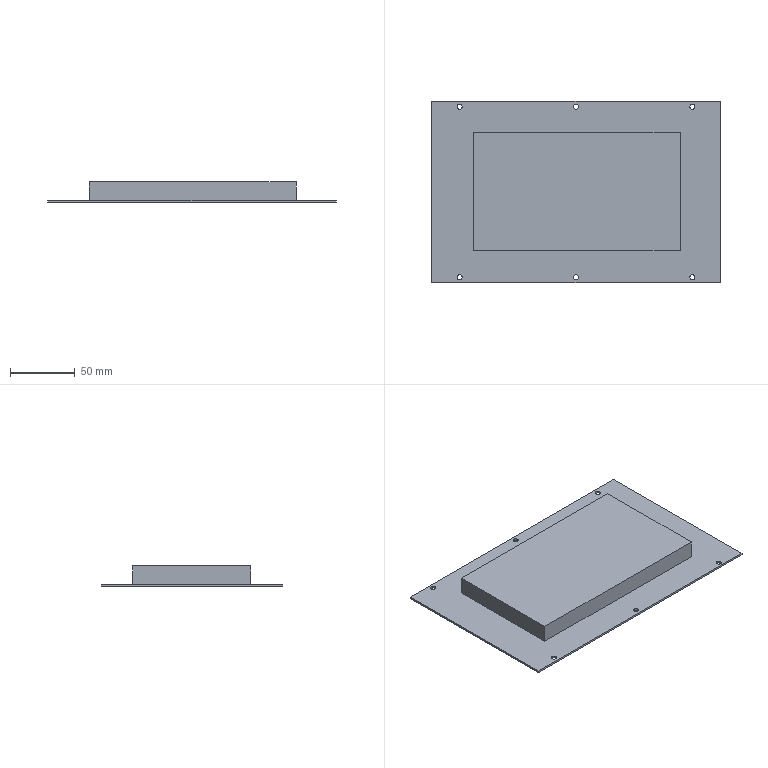Part | STEP file | Q7C1214W | 1 solid | 17 faces | box 223 x 140 x 15.5 mm | volume 251677 mm3 | plane 11 | cylinder 6 | commonest cylinder face diameters 4 x6
STEP:
#1=CARTESIAN_POINT('',(0.,0.,0.));
#2=DIRECTION('',(0.,0.,1.));
#3=DIRECTION('',(1.,0.,0.));
#4=AXIS2_PLACEMENT_3D('',#1,#2,#3);
#5=CARTESIAN_POINT('',(-79.5,46.,1.5));
#6=VERTEX_POINT('',#5);
#7=CARTESIAN_POINT('',(80.5,46.,1.5));
#8=VERTEX_POINT('',#7);
#9=CARTESIAN_POINT('',(-111.5,46.,1.5));
#10=DIRECTION('',(1.,0.,0.));
#11=VECTOR('',#10,1.);
#12=LINE('',#9,#11);
#13=CARTESIAN_POINT('',(-111.5,70.,1.5));
#14=DIRECTION('',(0.,0.,-1.));
#15=DIRECTION('',(-1.,0.,0.));
#16=AXIS2_PLACEMENT_3D('',#13,#14,#15);
#17=PLANE('',#16);
#18=CARTESIAN_POINT('',(0.,-24.));
#19=DIRECTION('',(-1.,0.));
#20=VECTOR('',#19,1.);
#21=LINE('',#18,#20);
#22=(GEOMETRIC_REPRESENTATION_CONTEXT(2)PARAMETRIC_REPRESENTATION_CONTEXT()REPRESENTATION_CONTEXT('',''));
#23=DEFINITIONAL_REPRESENTATION('',(#21),#22);
#24=PCURVE('',#17,#23);
#25=CARTESIAN_POINT('',(80.5,46.,15.5));
#26=DIRECTION('',(0.,1.,0.));
#27=DIRECTION('',(-1.,0.,0.));
#28=AXIS2_PLACEMENT_3D('',#25,#26,#27);
#29=PLANE('',#28);
#30=CARTESIAN_POINT('',(192.,-14.));
#31=DIRECTION('',(-1.,0.));
#32=VECTOR('',#31,1.);
#33=LINE('',#30,#32);
#34=(GEOMETRIC_REPRESENTATION_CONTEXT(2)PARAMETRIC_REPRESENTATION_CONTEXT()REPRESENTATION_CONTEXT('',''));
#35=DEFINITIONAL_REPRESENTATION('',(#33),#34);
#36=PCURVE('',#29,#35);
#37=SURFACE_CURVE('',#12,(#24,#36),.PCURVE_S1.);
#38=EDGE_CURVE('',#6,#8,#37,.T.);
#39=ORIENTED_EDGE('',*,*,#38,.T.);
#40=CARTESIAN_POINT('',(80.5,-45.5,1.5));
#41=VERTEX_POINT('',#40);
#42=CARTESIAN_POINT('',(80.5,70.,1.5));
#43=DIRECTION('',(0.,-1.,0.));
#44=VECTOR('',#43,1.);
#45=LINE('',#42,#44);
#46=CARTESIAN_POINT('',(-192.,0.));
#47=DIRECTION('',(0.,-1.));
#48=VECTOR('',#47,1.);
#49=LINE('',#46,#48);
#50=(GEOMETRIC_REPRESENTATION_CONTEXT(2)PARAMETRIC_REPRESENTATION_CONTEXT()REPRESENTATION_CONTEXT('',''));
#51=DEFINITIONAL_REPRESENTATION('',(#49),#50);
#52=PCURVE('',#17,#51);
#53=CARTESIAN_POINT('',(80.5,46.,15.5));
#54=DIRECTION('',(1.,0.,0.));
#55=DIRECTION('',(0.,1.,0.));
#56=AXIS2_PLACEMENT_3D('',#53,#54,#55);
#57=PLANE('',#56);
#58=CARTESIAN_POINT('',(24.,-14.));
#59=DIRECTION('',(-1.,0.));
#60=VECTOR('',#59,1.);
#61=LINE('',#58,#60);
#62=(GEOMETRIC_REPRESENTATION_CONTEXT(2)PARAMETRIC_REPRESENTATION_CONTEXT()REPRESENTATION_CONTEXT('',''));
#63=DEFINITIONAL_REPRESENTATION('',(#61),#62);
#64=PCURVE('',#57,#63);
#65=SURFACE_CURVE('',#45,(#52,#64),.PCURVE_S1.);
#66=EDGE_CURVE('',#8,#41,#65,.T.);
#67=ORIENTED_EDGE('',*,*,#66,.T.);
#68=CARTESIAN_POINT('',(-79.5,-45.5,1.5));
#69=VERTEX_POINT('',#68);
#70=CARTESIAN_POINT('',(-111.5,-45.5,1.5));
#71=DIRECTION('',(-1.,0.,0.));
#72=VECTOR('',#71,1.);
#73=LINE('',#70,#72);
#74=CARTESIAN_POINT('',(0.,-115.5));
#75=DIRECTION('',(1.,0.));
#76=VECTOR('',#75,1.);
#77=LINE('',#74,#76);
#78=(GEOMETRIC_REPRESENTATION_CONTEXT(2)PARAMETRIC_REPRESENTATION_CONTEXT()REPRESENTATION_CONTEXT('',''));
#79=DEFINITIONAL_REPRESENTATION('',(#77),#78);
#80=PCURVE('',#17,#79);
#81=CARTESIAN_POINT('',(80.5,-45.5,15.5));
#82=DIRECTION('',(0.,-1.,0.));
#83=DIRECTION('',(1.,0.,0.));
#84=AXIS2_PLACEMENT_3D('',#81,#82,#83);
#85=PLANE('',#84);
#86=CARTESIAN_POINT('',(-192.,-14.));
#87=DIRECTION('',(-1.,0.));
#88=VECTOR('',#87,1.);
#89=LINE('',#86,#88);
#90=(GEOMETRIC_REPRESENTATION_CONTEXT(2)PARAMETRIC_REPRESENTATION_CONTEXT()REPRESENTATION_CONTEXT('',''));
#91=DEFINITIONAL_REPRESENTATION('',(#89),#90);
#92=PCURVE('',#85,#91);
#93=SURFACE_CURVE('',#73,(#80,#92),.PCURVE_S1.);
#94=EDGE_CURVE('',#41,#69,#93,.T.);
#95=ORIENTED_EDGE('',*,*,#94,.T.);
#96=CARTESIAN_POINT('',(-79.5,70.,1.5));
#97=DIRECTION('',(0.,1.,0.));
#98=VECTOR('',#97,1.);
#99=LINE('',#96,#98);
#100=CARTESIAN_POINT('',(-32.,0.));
#101=DIRECTION('',(0.,1.));
#102=VECTOR('',#101,1.);
#103=LINE('',#100,#102);
#104=(GEOMETRIC_REPRESENTATION_CONTEXT(2)PARAMETRIC_REPRESENTATION_CONTEXT()REPRESENTATION_CONTEXT('',''));
#105=DEFINITIONAL_REPRESENTATION('',(#103),#104);
#106=PCURVE('',#17,#105);
#107=CARTESIAN_POINT('',(-79.5,46.,15.5));
#108=DIRECTION('',(-1.,0.,0.));
#109=DIRECTION('',(0.,-1.,0.));
#110=AXIS2_PLACEMENT_3D('',#107,#108,#109);
#111=PLANE('',#110);
#112=CARTESIAN_POINT('',(-24.,-14.));
#113=DIRECTION('',(-1.,0.));
#114=VECTOR('',#113,1.);
#115=LINE('',#112,#114);
#116=(GEOMETRIC_REPRESENTATION_CONTEXT(2)PARAMETRIC_REPRESENTATION_CONTEXT()REPRESENTATION_CONTEXT('',''));
#117=DEFINITIONAL_REPRESENTATION('',(#115),#116);
#118=PCURVE('',#111,#117);
#119=SURFACE_CURVE('',#99,(#106,#118),.PCURVE_S1.);
#120=EDGE_CURVE('',#69,#6,#119,.T.);
#121=ORIENTED_EDGE('',*,*,#120,.T.);
#122=EDGE_LOOP('',(#39,#67,#95,#121));
#123=FACE_BOUND('',#122,.T.);
#124=CARTESIAN_POINT('',(2.,-66.,1.5));
#125=VERTEX_POINT('',#124);
#126=CARTESIAN_POINT('',(0.,-66.,1.5));
#127=DIRECTION('',(0.,0.,1.));
#128=DIRECTION('',(1.,0.,0.));
#129=AXIS2_PLACEMENT_3D('',#126,#127,#128);
#130=CIRCLE('',#129,2.);
#131=CARTESIAN_POINT('',(-113.5,-136.));
#132=CARTESIAN_POINT('',(-113.5,-132.536));
#133=CARTESIAN_POINT('',(-110.5,-134.268));
#134=CARTESIAN_POINT('',(-107.5,-136.));
#135=CARTESIAN_POINT('',(-110.5,-137.732));
#136=CARTESIAN_POINT('',(-113.5,-139.464));
#137=CARTESIAN_POINT('',(-113.5,-136.));
#138=(BOUNDED_CURVE()B_SPLINE_CURVE(2,(#131,#132,#133,#134,#135,#136,#137),.UNSPECIFIED.,.T.,.F.)B_SPLINE_CURVE_WITH_KNOTS((1,2,2,2,2,1),(-2.094,0.,2.094,4.189,6.283,8.378),.UNSPECIFIED.)CURVE()GEOMETRIC_REPRESENTATION_ITEM()RATIONAL_B_SPLINE_CURVE((1.,0.5,1.,0.5,1.,0.5,1.))REPRESENTATION_ITEM(''));
#139=(GEOMETRIC_REPRESENTATION_CONTEXT(2)PARAMETRIC_REPRESENTATION_CONTEXT()REPRESENTATION_CONTEXT('',''));
#140=DEFINITIONAL_REPRESENTATION('',(#138),#139);
#141=PCURVE('',#17,#140);
#142=CARTESIAN_POINT('',(0.,-66.,1.5));
#143=DIRECTION('',(0.,0.,-1.));
#144=DIRECTION('',(-1.,0.,0.));
#145=AXIS2_PLACEMENT_3D('',#142,#143,#144);
#146=CYLINDRICAL_SURFACE('',#145,2.);
#147=CARTESIAN_POINT('',(9.425,0.));
#148=DIRECTION('',(-1.,0.));
#149=VECTOR('',#148,1.);
#150=LINE('',#147,#149);
#151=(GEOMETRIC_REPRESENTATION_CONTEXT(2)PARAMETRIC_REPRESENTATION_CONTEXT()REPRESENTATION_CONTEXT('',''));
#152=DEFINITIONAL_REPRESENTATION('',(#150),#151);
#153=PCURVE('',#146,#152);
#154=SURFACE_CURVE('',#130,(#141,#153),.PCURVE_S1.);
#155=EDGE_CURVE('',#125,#125,#154,.T.);
#156=ORIENTED_EDGE('',*,*,#155,.F.);
#157=EDGE_LOOP('',(#156));
#158=FACE_BOUND('',#157,.T.);
#159=CARTESIAN_POINT('',(92.,66.,1.5));
#160=VERTEX_POINT('',#159);
#161=CARTESIAN_POINT('',(90.,66.,1.5));
#162=DIRECTION('',(0.,0.,1.));
#163=DIRECTION('',(1.,0.,0.));
#164=AXIS2_PLACEMENT_3D('',#161,#162,#163);
#165=CIRCLE('',#164,2.);
#166=CARTESIAN_POINT('',(-203.5,-4.));
#167=CARTESIAN_POINT('',(-203.5,-0.5359));
#168=CARTESIAN_POINT('',(-200.5,-2.268));
#169=CARTESIAN_POINT('',(-197.5,-4.));
#170=CARTESIAN_POINT('',(-200.5,-5.732));
#171=CARTESIAN_POINT('',(-203.5,-7.464));
#172=CARTESIAN_POINT('',(-203.5,-4.));
#173=(BOUNDED_CURVE()B_SPLINE_CURVE(2,(#166,#167,#168,#169,#170,#171,#172),.UNSPECIFIED.,.T.,.F.)B_SPLINE_CURVE_WITH_KNOTS((1,2,2,2,2,1),(-2.094,0.,2.094,4.189,6.283,8.378),.UNSPECIFIED.)CURVE()GEOMETRIC_REPRESENTATION_ITEM()RATIONAL_B_SPLINE_CURVE((1.,0.5,1.,0.5,1.,0.5,1.))REPRESENTATION_ITEM(''));
#174=(GEOMETRIC_REPRESENTATION_CONTEXT(2)PARAMETRIC_REPRESENTATION_CONTEXT()REPRESENTATION_CONTEXT('',''));
#175=DEFINITIONAL_REPRESENTATION('',(#173),#174);
#176=PCURVE('',#17,#175);
#177=CARTESIAN_POINT('',(90.,66.,1.5));
#178=DIRECTION('',(0.,0.,-1.));
#179=DIRECTION('',(-1.,0.,0.));
#180=AXIS2_PLACEMENT_3D('',#177,#178,#179);
#181=CYLINDRICAL_SURFACE('',#180,2.);
#182=CARTESIAN_POINT('',(9.425,0.));
#183=DIRECTION('',(-1.,0.));
#184=VECTOR('',#183,1.);
#185=LINE('',#182,#184);
#186=(GEOMETRIC_REPRESENTATION_CONTEXT(2)PARAMETRIC_REPRESENTATION_CONTEXT()REPRESENTATION_CONTEXT('',''));
#187=DEFINITIONAL_REPRESENTATION('',(#185),#186);
#188=PCURVE('',#181,#187);
#189=SURFACE_CURVE('',#165,(#176,#188),.PCURVE_S1.);
#190=EDGE_CURVE('',#160,#160,#189,.T.);
#191=ORIENTED_EDGE('',*,*,#190,.F.);
#192=EDGE_LOOP('',(#191));
#193=FACE_BOUND('',#192,.T.);
#194=CARTESIAN_POINT('',(-88.,66.,1.5));
#195=VERTEX_POINT('',#194);
#196=CARTESIAN_POINT('',(-90.,66.,1.5));
#197=DIRECTION('',(0.,0.,1.));
#198=DIRECTION('',(1.,0.,0.));
#199=AXIS2_PLACEMENT_3D('',#196,#197,#198);
#200=CIRCLE('',#199,2.);
#201=CARTESIAN_POINT('',(-23.5,-4.));
#202=CARTESIAN_POINT('',(-23.5,-0.5359));
#203=CARTESIAN_POINT('',(-20.5,-2.268));
#204=CARTESIAN_POINT('',(-17.5,-4.));
#205=CARTESIAN_POINT('',(-20.5,-5.732));
#206=CARTESIAN_POINT('',(-23.5,-7.464));
#207=CARTESIAN_POINT('',(-23.5,-4.));
#208=(BOUNDED_CURVE()B_SPLINE_CURVE(2,(#201,#202,#203,#204,#205,#206,#207),.UNSPECIFIED.,.T.,.F.)B_SPLINE_CURVE_WITH_KNOTS((1,2,2,2,2,1),(-2.094,0.,2.094,4.189,6.283,8.378),.UNSPECIFIED.)CURVE()GEOMETRIC_REPRESENTATION_ITEM()RATIONAL_B_SPLINE_CURVE((1.,0.5,1.,0.5,1.,0.5,1.))REPRESENTATION_ITEM(''));
#209=(GEOMETRIC_REPRESENTATION_CONTEXT(2)PARAMETRIC_REPRESENTATION_CONTEXT()REPRESENTATION_CONTEXT('',''));
#210=DEFINITIONAL_REPRESENTATION('',(#208),#209);
#211=PCURVE('',#17,#210);
#212=CARTESIAN_POINT('',(-90.,66.,1.5));
#213=DIRECTION('',(0.,0.,-1.));
#214=DIRECTION('',(-1.,0.,0.));
#215=AXIS2_PLACEMENT_3D('',#212,#213,#214);
#216=CYLINDRICAL_SURFACE('',#215,2.);
#217=CARTESIAN_POINT('',(9.425,0.));
#218=DIRECTION('',(-1.,0.));
#219=VECTOR('',#218,1.);
#220=LINE('',#217,#219);
#221=(GEOMETRIC_REPRESENTATION_CONTEXT(2)PARAMETRIC_REPRESENTATION_CONTEXT()REPRESENTATION_CONTEXT('',''));
#222=DEFINITIONAL_REPRESENTATION('',(#220),#221);
#223=PCURVE('',#216,#222);
#224=SURFACE_CURVE('',#200,(#211,#223),.PCURVE_S1.);
#225=EDGE_CURVE('',#195,#195,#224,.T.);
#226=ORIENTED_EDGE('',*,*,#225,.F.);
#227=EDGE_LOOP('',(#226));
#228=FACE_BOUND('',#227,.T.);
#229=CARTESIAN_POINT('',(-111.5,70.,1.5));
#230=VERTEX_POINT('',#229);
#231=CARTESIAN_POINT('',(-111.5,-70.,1.5));
#232=VERTEX_POINT('',#231);
#233=CARTESIAN_POINT('',(-111.5,-70.,1.5));
#234=DIRECTION('',(0.,-1.,0.));
#235=VECTOR('',#234,1.);
#236=LINE('',#233,#235);
#237=CARTESIAN_POINT('',(0.,-140.));
#238=DIRECTION('',(0.,-1.));
#239=VECTOR('',#238,1.);
#240=LINE('',#237,#239);
#241=(GEOMETRIC_REPRESENTATION_CONTEXT(2)PARAMETRIC_REPRESENTATION_CONTEXT()REPRESENTATION_CONTEXT('',''));
#242=DEFINITIONAL_REPRESENTATION('',(#240),#241);
#243=PCURVE('',#17,#242);
#244=CARTESIAN_POINT('',(-111.5,-70.,1.5));
#245=DIRECTION('',(1.,0.,0.));
#246=DIRECTION('',(0.,0.,-1.));
#247=AXIS2_PLACEMENT_3D('',#244,#245,#246);
#248=PLANE('',#247);
#249=CARTESIAN_POINT('',(0.,0.));
#250=DIRECTION('',(0.,-1.));
#251=VECTOR('',#250,1.);
#252=LINE('',#249,#251);
#253=(GEOMETRIC_REPRESENTATION_CONTEXT(2)PARAMETRIC_REPRESENTATION_CONTEXT()REPRESENTATION_CONTEXT('',''));
#254=DEFINITIONAL_REPRESENTATION('',(#252),#253);
#255=PCURVE('',#248,#254);
#256=SURFACE_CURVE('',#236,(#243,#255),.PCURVE_S1.);
#257=EDGE_CURVE('',#230,#232,#256,.T.);
#258=ORIENTED_EDGE('',*,*,#257,.T.);
#259=CARTESIAN_POINT('',(111.5,-70.,1.5));
#260=VERTEX_POINT('',#259);
#261=CARTESIAN_POINT('',(-111.5,-70.,1.5));
#262=DIRECTION('',(1.,0.,0.));
#263=VECTOR('',#262,1.);
#264=LINE('',#261,#263);
#265=CARTESIAN_POINT('',(0.,-140.));
#266=DIRECTION('',(-1.,0.));
#267=VECTOR('',#266,1.);
#268=LINE('',#265,#267);
#269=(GEOMETRIC_REPRESENTATION_CONTEXT(2)PARAMETRIC_REPRESENTATION_CONTEXT()REPRESENTATION_CONTEXT('',''));
#270=DEFINITIONAL_REPRESENTATION('',(#268),#269);
#271=PCURVE('',#17,#270);
#272=CARTESIAN_POINT('',(-111.5,-70.,1.5));
#273=DIRECTION('',(0.,1.,0.));
#274=DIRECTION('',(0.,0.,1.));
#275=AXIS2_PLACEMENT_3D('',#272,#273,#274);
#276=PLANE('',#275);
#277=CARTESIAN_POINT('',(0.,0.));
#278=DIRECTION('',(0.,1.));
#279=VECTOR('',#278,1.);
#280=LINE('',#277,#279);
#281=(GEOMETRIC_REPRESENTATION_CONTEXT(2)PARAMETRIC_REPRESENTATION_CONTEXT()REPRESENTATION_CONTEXT('',''));
#282=DEFINITIONAL_REPRESENTATION('',(#280),#281);
#283=PCURVE('',#276,#282);
#284=SURFACE_CURVE('',#264,(#271,#283),.PCURVE_S1.);
#285=EDGE_CURVE('',#232,#260,#284,.T.);
#286=ORIENTED_EDGE('',*,*,#285,.T.);
#287=CARTESIAN_POINT('',(111.5,70.,1.5));
#288=VERTEX_POINT('',#287);
#289=CARTESIAN_POINT('',(111.5,-70.,1.5));
#290=DIRECTION('',(0.,1.,0.));
#291=VECTOR('',#290,1.);
#292=LINE('',#289,#291);
#293=CARTESIAN_POINT('',(-223.,-140.));
#294=DIRECTION('',(0.,1.));
#295=VECTOR('',#294,1.);
#296=LINE('',#293,#295);
#297=(GEOMETRIC_REPRESENTATION_CONTEXT(2)PARAMETRIC_REPRESENTATION_CONTEXT()REPRESENTATION_CONTEXT('',''));
#298=DEFINITIONAL_REPRESENTATION('',(#296),#297);
#299=PCURVE('',#17,#298);
#300=CARTESIAN_POINT('',(111.5,-70.,1.5));
#301=DIRECTION('',(-1.,0.,0.));
#302=DIRECTION('',(0.,0.,1.));
#303=AXIS2_PLACEMENT_3D('',#300,#301,#302);
#304=PLANE('',#303);
#305=CARTESIAN_POINT('',(0.,0.));
#306=DIRECTION('',(0.,1.));
#307=VECTOR('',#306,1.);
#308=LINE('',#305,#307);
#309=(GEOMETRIC_REPRESENTATION_CONTEXT(2)PARAMETRIC_REPRESENTATION_CONTEXT()REPRESENTATION_CONTEXT('',''));
#310=DEFINITIONAL_REPRESENTATION('',(#308),#309);
#311=PCURVE('',#304,#310);
#312=SURFACE_CURVE('',#292,(#299,#311),.PCURVE_S1.);
#313=EDGE_CURVE('',#260,#288,#312,.T.);
#314=ORIENTED_EDGE('',*,*,#313,.T.);
#315=CARTESIAN_POINT('',(-111.5,70.,1.5));
#316=DIRECTION('',(-1.,0.,0.));
#317=VECTOR('',#316,1.);
#318=LINE('',#315,#317);
#319=CARTESIAN_POINT('',(0.,0.));
#320=DIRECTION('',(1.,0.));
#321=VECTOR('',#320,1.);
#322=LINE('',#319,#321);
#323=(GEOMETRIC_REPRESENTATION_CONTEXT(2)PARAMETRIC_REPRESENTATION_CONTEXT()REPRESENTATION_CONTEXT('',''));
#324=DEFINITIONAL_REPRESENTATION('',(#322),#323);
#325=PCURVE('',#17,#324);
#326=CARTESIAN_POINT('',(-111.5,70.,1.5));
#327=DIRECTION('',(0.,-1.,0.));
#328=DIRECTION('',(0.,0.,-1.));
#329=AXIS2_PLACEMENT_3D('',#326,#327,#328);
#330=PLANE('',#329);
#331=CARTESIAN_POINT('',(0.,0.));
#332=DIRECTION('',(0.,-1.));
#333=VECTOR('',#332,1.);
#334=LINE('',#331,#333);
#335=(GEOMETRIC_REPRESENTATION_CONTEXT(2)PARAMETRIC_REPRESENTATION_CONTEXT()REPRESENTATION_CONTEXT('',''));
#336=DEFINITIONAL_REPRESENTATION('',(#334),#335);
#337=PCURVE('',#330,#336);
#338=SURFACE_CURVE('',#318,(#325,#337),.PCURVE_S1.);
#339=EDGE_CURVE('',#288,#230,#338,.T.);
#340=ORIENTED_EDGE('',*,*,#339,.T.);
#341=EDGE_LOOP('',(#258,#286,#314,#340));
#342=FACE_BOUND('',#341,.T.);
#343=CARTESIAN_POINT('',(2.,66.,1.5));
#344=VERTEX_POINT('',#343);
#345=CARTESIAN_POINT('',(0.,66.,1.5));
#346=DIRECTION('',(0.,0.,1.));
#347=DIRECTION('',(1.,0.,0.));
#348=AXIS2_PLACEMENT_3D('',#345,#346,#347);
#349=CIRCLE('',#348,2.);
#350=CARTESIAN_POINT('',(-113.5,-4.));
#351=CARTESIAN_POINT('',(-113.5,-0.5359));
#352=CARTESIAN_POINT('',(-110.5,-2.268));
#353=CARTESIAN_POINT('',(-107.5,-4.));
#354=CARTESIAN_POINT('',(-110.5,-5.732));
#355=CARTESIAN_POINT('',(-113.5,-7.464));
#356=CARTESIAN_POINT('',(-113.5,-4.));
#357=(BOUNDED_CURVE()B_SPLINE_CURVE(2,(#350,#351,#352,#353,#354,#355,#356),.UNSPECIFIED.,.T.,.F.)B_SPLINE_CURVE_WITH_KNOTS((1,2,2,2,2,1),(-2.094,0.,2.094,4.189,6.283,8.378),.UNSPECIFIED.)CURVE()GEOMETRIC_REPRESENTATION_ITEM()RATIONAL_B_SPLINE_CURVE((1.,0.5,1.,0.5,1.,0.5,1.))REPRESENTATION_ITEM(''));
#358=(GEOMETRIC_REPRESENTATION_CONTEXT(2)PARAMETRIC_REPRESENTATION_CONTEXT()REPRESENTATION_CONTEXT('',''));
#359=DEFINITIONAL_REPRESENTATION('',(#357),#358);
#360=PCURVE('',#17,#359);
#361=CARTESIAN_POINT('',(0.,66.,1.5));
#362=DIRECTION('',(0.,0.,-1.));
#363=DIRECTION('',(-1.,0.,0.));
#364=AXIS2_PLACEMENT_3D('',#361,#362,#363);
#365=CYLINDRICAL_SURFACE('',#364,2.);
#366=CARTESIAN_POINT('',(9.425,0.));
#367=DIRECTION('',(-1.,0.));
#368=VECTOR('',#367,1.);
#369=LINE('',#366,#368);
#370=(GEOMETRIC_REPRESENTATION_CONTEXT(2)PARAMETRIC_REPRESENTATION_CONTEXT()REPRESENTATION_CONTEXT('',''));
#371=DEFINITIONAL_REPRESENTATION('',(#369),#370);
#372=PCURVE('',#365,#371);
#373=SURFACE_CURVE('',#349,(#360,#372),.PCURVE_S1.);
#374=EDGE_CURVE('',#344,#344,#373,.T.);
#375=ORIENTED_EDGE('',*,*,#374,.F.);
#376=EDGE_LOOP('',(#375));
#377=FACE_BOUND('',#376,.T.);
#378=CARTESIAN_POINT('',(-88.,-66.,1.5));
#379=VERTEX_POINT('',#378);
#380=CARTESIAN_POINT('',(-90.,-66.,1.5));
#381=DIRECTION('',(0.,0.,1.));
#382=DIRECTION('',(1.,0.,0.));
#383=AXIS2_PLACEMENT_3D('',#380,#381,#382);
#384=CIRCLE('',#383,2.);
#385=CARTESIAN_POINT('',(-23.5,-136.));
#386=CARTESIAN_POINT('',(-23.5,-132.536));
#387=CARTESIAN_POINT('',(-20.5,-134.268));
#388=CARTESIAN_POINT('',(-17.5,-136.));
#389=CARTESIAN_POINT('',(-20.5,-137.732));
#390=CARTESIAN_POINT('',(-23.5,-139.464));
#391=CARTESIAN_POINT('',(-23.5,-136.));
#392=(BOUNDED_CURVE()B_SPLINE_CURVE(2,(#385,#386,#387,#388,#389,#390,#391),.UNSPECIFIED.,.T.,.F.)B_SPLINE_CURVE_WITH_KNOTS((1,2,2,2,2,1),(-2.094,0.,2.094,4.189,6.283,8.378),.UNSPECIFIED.)CURVE()GEOMETRIC_REPRESENTATION_ITEM()RATIONAL_B_SPLINE_CURVE((1.,0.5,1.,0.5,1.,0.5,1.))REPRESENTATION_ITEM(''));
#393=(GEOMETRIC_REPRESENTATION_CONTEXT(2)PARAMETRIC_REPRESENTATION_CONTEXT()REPRESENTATION_CONTEXT('',''));
#394=DEFINITIONAL_REPRESENTATION('',(#392),#393);
#395=PCURVE('',#17,#394);
#396=CARTESIAN_POINT('',(-90.,-66.,1.5));
#397=DIRECTION('',(0.,0.,-1.));
#398=DIRECTION('',(-1.,0.,0.));
#399=AXIS2_PLACEMENT_3D('',#396,#397,#398);
#400=CYLINDRICAL_SURFACE('',#399,2.);
#401=CARTESIAN_POINT('',(9.425,0.));
#402=DIRECTION('',(-1.,0.));
#403=VECTOR('',#402,1.);
#404=LINE('',#401,#403);
#405=(GEOMETRIC_REPRESENTATION_CONTEXT(2)PARAMETRIC_REPRESENTATION_CONTEXT()REPRESENTATION_CONTEXT('',''));
#406=DEFINITIONAL_REPRESENTATION('',(#404),#405);
#407=PCURVE('',#400,#406);
#408=SURFACE_CURVE('',#384,(#395,#407),.PCURVE_S1.);
#409=EDGE_CURVE('',#379,#379,#408,.T.);
#410=ORIENTED_EDGE('',*,*,#409,.F.);
#411=EDGE_LOOP('',(#410));
#412=FACE_BOUND('',#411,.T.);
#413=CARTESIAN_POINT('',(92.,-66.,1.5));
#414=VERTEX_POINT('',#413);
#415=CARTESIAN_POINT('',(90.,-66.,1.5));
#416=DIRECTION('',(0.,0.,1.));
#417=DIRECTION('',(1.,0.,0.));
#418=AXIS2_PLACEMENT_3D('',#415,#416,#417);
#419=CIRCLE('',#418,2.);
#420=CARTESIAN_POINT('',(-203.5,-136.));
#421=CARTESIAN_POINT('',(-203.5,-132.536));
#422=CARTESIAN_POINT('',(-200.5,-134.268));
#423=CARTESIAN_POINT('',(-197.5,-136.));
#424=CARTESIAN_POINT('',(-200.5,-137.732));
#425=CARTESIAN_POINT('',(-203.5,-139.464));
#426=CARTESIAN_POINT('',(-203.5,-136.));
#427=(BOUNDED_CURVE()B_SPLINE_CURVE(2,(#420,#421,#422,#423,#424,#425,#426),.UNSPECIFIED.,.T.,.F.)B_SPLINE_CURVE_WITH_KNOTS((1,2,2,2,2,1),(-2.094,0.,2.094,4.189,6.283,8.378),.UNSPECIFIED.)CURVE()GEOMETRIC_REPRESENTATION_ITEM()RATIONAL_B_SPLINE_CURVE((1.,0.5,1.,0.5,1.,0.5,1.))REPRESENTATION_ITEM(''));
#428=(GEOMETRIC_REPRESENTATION_CONTEXT(2)PARAMETRIC_REPRESENTATION_CONTEXT()REPRESENTATION_CONTEXT('',''));
#429=DEFINITIONAL_REPRESENTATION('',(#427),#428);
#430=PCURVE('',#17,#429);
#431=CARTESIAN_POINT('',(90.,-66.,1.5));
#432=DIRECTION('',(0.,0.,-1.));
#433=DIRECTION('',(-1.,0.,0.));
#434=AXIS2_PLACEMENT_3D('',#431,#432,#433);
#435=CYLINDRICAL_SURFACE('',#434,2.);
#436=CARTESIAN_POINT('',(9.425,0.));
#437=DIRECTION('',(-1.,0.));
#438=VECTOR('',#437,1.);
#439=LINE('',#436,#438);
#440=(GEOMETRIC_REPRESENTATION_CONTEXT(2)PARAMETRIC_REPRESENTATION_CONTEXT()REPRESENTATION_CONTEXT('',''));
#441=DEFINITIONAL_REPRESENTATION('',(#439),#440);
#442=PCURVE('',#435,#441);
#443=SURFACE_CURVE('',#419,(#430,#442),.PCURVE_S1.);
#444=EDGE_CURVE('',#414,#414,#443,.T.);
#445=ORIENTED_EDGE('',*,*,#444,.F.);
#446=EDGE_LOOP('',(#445));
#447=FACE_BOUND('',#446,.T.);
#448=ADVANCED_FACE('',(#123,#158,#193,#228,#342,#377,#412,#447),#17,.F.);
#449=CARTESIAN_POINT('',(2.,-66.,0.));
#450=VERTEX_POINT('',#449);
#451=CARTESIAN_POINT('',(0.,-66.,0.));
#452=DIRECTION('',(0.,0.,1.));
#453=DIRECTION('',(1.,0.,0.));
#454=AXIS2_PLACEMENT_3D('',#451,#452,#453);
#455=CIRCLE('',#454,2.);
#456=CARTESIAN_POINT('',(-111.5,70.,0.));
#457=DIRECTION('',(0.,0.,-1.));
#458=DIRECTION('',(-1.,0.,0.));
#459=AXIS2_PLACEMENT_3D('',#456,#457,#458);
#460=PLANE('',#459);
#461=CARTESIAN_POINT('',(-113.5,-136.));
#462=CARTESIAN_POINT('',(-113.5,-132.536));
#463=CARTESIAN_POINT('',(-110.5,-134.268));
#464=CARTESIAN_POINT('',(-107.5,-136.));
#465=CARTESIAN_POINT('',(-110.5,-137.732));
#466=CARTESIAN_POINT('',(-113.5,-139.464));
#467=CARTESIAN_POINT('',(-113.5,-136.));
#468=(BOUNDED_CURVE()B_SPLINE_CURVE(2,(#461,#462,#463,#464,#465,#466,#467),.UNSPECIFIED.,.T.,.F.)B_SPLINE_CURVE_WITH_KNOTS((1,2,2,2,2,1),(-2.094,0.,2.094,4.189,6.283,8.378),.UNSPECIFIED.)CURVE()GEOMETRIC_REPRESENTATION_ITEM()RATIONAL_B_SPLINE_CURVE((1.,0.5,1.,0.5,1.,0.5,1.))REPRESENTATION_ITEM(''));
#469=(GEOMETRIC_REPRESENTATION_CONTEXT(2)PARAMETRIC_REPRESENTATION_CONTEXT()REPRESENTATION_CONTEXT('',''));
#470=DEFINITIONAL_REPRESENTATION('',(#468),#469);
#471=PCURVE('',#460,#470);
#472=CARTESIAN_POINT('',(9.425,1.5));
#473=DIRECTION('',(-1.,0.));
#474=VECTOR('',#473,1.);
#475=LINE('',#472,#474);
#476=(GEOMETRIC_REPRESENTATION_CONTEXT(2)PARAMETRIC_REPRESENTATION_CONTEXT()REPRESENTATION_CONTEXT('',''));
#477=DEFINITIONAL_REPRESENTATION('',(#475),#476);
#478=PCURVE('',#146,#477);
#479=SURFACE_CURVE('',#455,(#471,#478),.PCURVE_S1.);
#480=EDGE_CURVE('',#450,#450,#479,.T.);
#481=ORIENTED_EDGE('',*,*,#480,.T.);
#482=EDGE_LOOP('',(#481));
#483=FACE_BOUND('',#482,.T.);
#484=CARTESIAN_POINT('',(92.,66.,0.));
#485=VERTEX_POINT('',#484);
#486=CARTESIAN_POINT('',(90.,66.,0.));
#487=DIRECTION('',(0.,0.,1.));
#488=DIRECTION('',(1.,0.,0.));
#489=AXIS2_PLACEMENT_3D('',#486,#487,#488);
#490=CIRCLE('',#489,2.);
#491=CARTESIAN_POINT('',(-203.5,-4.));
#492=CARTESIAN_POINT('',(-203.5,-0.5359));
#493=CARTESIAN_POINT('',(-200.5,-2.268));
#494=CARTESIAN_POINT('',(-197.5,-4.));
#495=CARTESIAN_POINT('',(-200.5,-5.732));
#496=CARTESIAN_POINT('',(-203.5,-7.464));
#497=CARTESIAN_POINT('',(-203.5,-4.));
#498=(BOUNDED_CURVE()B_SPLINE_CURVE(2,(#491,#492,#493,#494,#495,#496,#497),.UNSPECIFIED.,.T.,.F.)B_SPLINE_CURVE_WITH_KNOTS((1,2,2,2,2,1),(-2.094,0.,2.094,4.189,6.283,8.378),.UNSPECIFIED.)CURVE()GEOMETRIC_REPRESENTATION_ITEM()RATIONAL_B_SPLINE_CURVE((1.,0.5,1.,0.5,1.,0.5,1.))REPRESENTATION_ITEM(''));
#499=(GEOMETRIC_REPRESENTATION_CONTEXT(2)PARAMETRIC_REPRESENTATION_CONTEXT()REPRESENTATION_CONTEXT('',''));
#500=DEFINITIONAL_REPRESENTATION('',(#498),#499);
#501=PCURVE('',#460,#500);
#502=CARTESIAN_POINT('',(9.425,1.5));
#503=DIRECTION('',(-1.,0.));
#504=VECTOR('',#503,1.);
#505=LINE('',#502,#504);
#506=(GEOMETRIC_REPRESENTATION_CONTEXT(2)PARAMETRIC_REPRESENTATION_CONTEXT()REPRESENTATION_CONTEXT('',''));
#507=DEFINITIONAL_REPRESENTATION('',(#505),#506);
#508=PCURVE('',#181,#507);
#509=SURFACE_CURVE('',#490,(#501,#508),.PCURVE_S1.);
#510=EDGE_CURVE('',#485,#485,#509,.T.);
#511=ORIENTED_EDGE('',*,*,#510,.T.);
#512=EDGE_LOOP('',(#511));
#513=FACE_BOUND('',#512,.T.);
#514=CARTESIAN_POINT('',(-88.,66.,0.));
#515=VERTEX_POINT('',#514);
#516=CARTESIAN_POINT('',(-90.,66.,0.));
#517=DIRECTION('',(0.,0.,1.));
#518=DIRECTION('',(1.,0.,0.));
#519=AXIS2_PLACEMENT_3D('',#516,#517,#518);
#520=CIRCLE('',#519,2.);
#521=CARTESIAN_POINT('',(-23.5,-4.));
#522=CARTESIAN_POINT('',(-23.5,-0.5359));
#523=CARTESIAN_POINT('',(-20.5,-2.268));
#524=CARTESIAN_POINT('',(-17.5,-4.));
#525=CARTESIAN_POINT('',(-20.5,-5.732));
#526=CARTESIAN_POINT('',(-23.5,-7.464));
#527=CARTESIAN_POINT('',(-23.5,-4.));
#528=(BOUNDED_CURVE()B_SPLINE_CURVE(2,(#521,#522,#523,#524,#525,#526,#527),.UNSPECIFIED.,.T.,.F.)B_SPLINE_CURVE_WITH_KNOTS((1,2,2,2,2,1),(-2.094,0.,2.094,4.189,6.283,8.378),.UNSPECIFIED.)CURVE()GEOMETRIC_REPRESENTATION_ITEM()RATIONAL_B_SPLINE_CURVE((1.,0.5,1.,0.5,1.,0.5,1.))REPRESENTATION_ITEM(''));
#529=(GEOMETRIC_REPRESENTATION_CONTEXT(2)PARAMETRIC_REPRESENTATION_CONTEXT()REPRESENTATION_CONTEXT('',''));
#530=DEFINITIONAL_REPRESENTATION('',(#528),#529);
#531=PCURVE('',#460,#530);
#532=CARTESIAN_POINT('',(9.425,1.5));
#533=DIRECTION('',(-1.,0.));
#534=VECTOR('',#533,1.);
#535=LINE('',#532,#534);
#536=(GEOMETRIC_REPRESENTATION_CONTEXT(2)PARAMETRIC_REPRESENTATION_CONTEXT()REPRESENTATION_CONTEXT('',''));
#537=DEFINITIONAL_REPRESENTATION('',(#535),#536);
#538=PCURVE('',#216,#537);
#539=SURFACE_CURVE('',#520,(#531,#538),.PCURVE_S1.);
#540=EDGE_CURVE('',#515,#515,#539,.T.);
#541=ORIENTED_EDGE('',*,*,#540,.T.);
#542=EDGE_LOOP('',(#541));
#543=FACE_BOUND('',#542,.T.);
#544=CARTESIAN_POINT('',(-111.5,70.,0.));
#545=VERTEX_POINT('',#544);
#546=CARTESIAN_POINT('',(-111.5,-70.,0.));
#547=VERTEX_POINT('',#546);
#548=CARTESIAN_POINT('',(-111.5,-70.,0.));
#549=DIRECTION('',(0.,-1.,0.));
#550=VECTOR('',#549,1.);
#551=LINE('',#548,#550);
#552=CARTESIAN_POINT('',(0.,-140.));
#553=DIRECTION('',(0.,-1.));
#554=VECTOR('',#553,1.);
#555=LINE('',#552,#554);
#556=(GEOMETRIC_REPRESENTATION_CONTEXT(2)PARAMETRIC_REPRESENTATION_CONTEXT()REPRESENTATION_CONTEXT('',''));
#557=DEFINITIONAL_REPRESENTATION('',(#555),#556);
#558=PCURVE('',#460,#557);
#559=CARTESIAN_POINT('',(1.5,0.));
#560=DIRECTION('',(0.,-1.));
#561=VECTOR('',#560,1.);
#562=LINE('',#559,#561);
#563=(GEOMETRIC_REPRESENTATION_CONTEXT(2)PARAMETRIC_REPRESENTATION_CONTEXT()REPRESENTATION_CONTEXT('',''));
#564=DEFINITIONAL_REPRESENTATION('',(#562),#563);
#565=PCURVE('',#248,#564);
#566=SURFACE_CURVE('',#551,(#558,#565),.PCURVE_S1.);
#567=EDGE_CURVE('',#545,#547,#566,.T.);
#568=ORIENTED_EDGE('',*,*,#567,.F.);
#569=CARTESIAN_POINT('',(111.5,70.,0.));
#570=VERTEX_POINT('',#569);
#571=CARTESIAN_POINT('',(-111.5,70.,0.));
#572=DIRECTION('',(-1.,0.,0.));
#573=VECTOR('',#572,1.);
#574=LINE('',#571,#573);
#575=CARTESIAN_POINT('',(0.,0.));
#576=DIRECTION('',(1.,0.));
#577=VECTOR('',#576,1.);
#578=LINE('',#575,#577);
#579=(GEOMETRIC_REPRESENTATION_CONTEXT(2)PARAMETRIC_REPRESENTATION_CONTEXT()REPRESENTATION_CONTEXT('',''));
#580=DEFINITIONAL_REPRESENTATION('',(#578),#579);
#581=PCURVE('',#460,#580);
#582=CARTESIAN_POINT('',(1.5,0.));
#583=DIRECTION('',(0.,-1.));
#584=VECTOR('',#583,1.);
#585=LINE('',#582,#584);
#586=(GEOMETRIC_REPRESENTATION_CONTEXT(2)PARAMETRIC_REPRESENTATION_CONTEXT()REPRESENTATION_CONTEXT('',''));
#587=DEFINITIONAL_REPRESENTATION('',(#585),#586);
#588=PCURVE('',#330,#587);
#589=SURFACE_CURVE('',#574,(#581,#588),.PCURVE_S1.);
#590=EDGE_CURVE('',#570,#545,#589,.T.);
#591=ORIENTED_EDGE('',*,*,#590,.F.);
#592=CARTESIAN_POINT('',(111.5,-70.,0.));
#593=VERTEX_POINT('',#592);
#594=CARTESIAN_POINT('',(111.5,-70.,0.));
#595=DIRECTION('',(0.,1.,0.));
#596=VECTOR('',#595,1.);
#597=LINE('',#594,#596);
#598=CARTESIAN_POINT('',(-223.,-140.));
#599=DIRECTION('',(0.,1.));
#600=VECTOR('',#599,1.);
#601=LINE('',#598,#600);
#602=(GEOMETRIC_REPRESENTATION_CONTEXT(2)PARAMETRIC_REPRESENTATION_CONTEXT()REPRESENTATION_CONTEXT('',''));
#603=DEFINITIONAL_REPRESENTATION('',(#601),#602);
#604=PCURVE('',#460,#603);
#605=CARTESIAN_POINT('',(-1.5,0.));
#606=DIRECTION('',(0.,1.));
#607=VECTOR('',#606,1.);
#608=LINE('',#605,#607);
#609=(GEOMETRIC_REPRESENTATION_CONTEXT(2)PARAMETRIC_REPRESENTATION_CONTEXT()REPRESENTATION_CONTEXT('',''));
#610=DEFINITIONAL_REPRESENTATION('',(#608),#609);
#611=PCURVE('',#304,#610);
#612=SURFACE_CURVE('',#597,(#604,#611),.PCURVE_S1.);
#613=EDGE_CURVE('',#593,#570,#612,.T.);
#614=ORIENTED_EDGE('',*,*,#613,.F.);
#615=CARTESIAN_POINT('',(-111.5,-70.,0.));
#616=DIRECTION('',(1.,0.,0.));
#617=VECTOR('',#616,1.);
#618=LINE('',#615,#617);
#619=CARTESIAN_POINT('',(0.,-140.));
#620=DIRECTION('',(-1.,0.));
#621=VECTOR('',#620,1.);
#622=LINE('',#619,#621);
#623=(GEOMETRIC_REPRESENTATION_CONTEXT(2)PARAMETRIC_REPRESENTATION_CONTEXT()REPRESENTATION_CONTEXT('',''));
#624=DEFINITIONAL_REPRESENTATION('',(#622),#623);
#625=PCURVE('',#460,#624);
#626=CARTESIAN_POINT('',(-1.5,0.));
#627=DIRECTION('',(0.,1.));
#628=VECTOR('',#627,1.);
#629=LINE('',#626,#628);
#630=(GEOMETRIC_REPRESENTATION_CONTEXT(2)PARAMETRIC_REPRESENTATION_CONTEXT()REPRESENTATION_CONTEXT('',''));
#631=DEFINITIONAL_REPRESENTATION('',(#629),#630);
#632=PCURVE('',#276,#631);
#633=SURFACE_CURVE('',#618,(#625,#632),.PCURVE_S1.);
#634=EDGE_CURVE('',#547,#593,#633,.T.);
#635=ORIENTED_EDGE('',*,*,#634,.F.);
#636=EDGE_LOOP('',(#568,#591,#614,#635));
#637=FACE_BOUND('',#636,.T.);
#638=CARTESIAN_POINT('',(2.,66.,0.));
#639=VERTEX_POINT('',#638);
#640=CARTESIAN_POINT('',(0.,66.,0.));
#641=DIRECTION('',(0.,0.,1.));
#642=DIRECTION('',(1.,0.,0.));
#643=AXIS2_PLACEMENT_3D('',#640,#641,#642);
#644=CIRCLE('',#643,2.);
#645=CARTESIAN_POINT('',(-113.5,-4.));
#646=CARTESIAN_POINT('',(-113.5,-0.5359));
#647=CARTESIAN_POINT('',(-110.5,-2.268));
#648=CARTESIAN_POINT('',(-107.5,-4.));
#649=CARTESIAN_POINT('',(-110.5,-5.732));
#650=CARTESIAN_POINT('',(-113.5,-7.464));
#651=CARTESIAN_POINT('',(-113.5,-4.));
#652=(BOUNDED_CURVE()B_SPLINE_CURVE(2,(#645,#646,#647,#648,#649,#650,#651),.UNSPECIFIED.,.T.,.F.)B_SPLINE_CURVE_WITH_KNOTS((1,2,2,2,2,1),(-2.094,0.,2.094,4.189,6.283,8.378),.UNSPECIFIED.)CURVE()GEOMETRIC_REPRESENTATION_ITEM()RATIONAL_B_SPLINE_CURVE((1.,0.5,1.,0.5,1.,0.5,1.))REPRESENTATION_ITEM(''));
#653=(GEOMETRIC_REPRESENTATION_CONTEXT(2)PARAMETRIC_REPRESENTATION_CONTEXT()REPRESENTATION_CONTEXT('',''));
#654=DEFINITIONAL_REPRESENTATION('',(#652),#653);
#655=PCURVE('',#460,#654);
#656=CARTESIAN_POINT('',(9.425,1.5));
#657=DIRECTION('',(-1.,0.));
#658=VECTOR('',#657,1.);
#659=LINE('',#656,#658);
#660=(GEOMETRIC_REPRESENTATION_CONTEXT(2)PARAMETRIC_REPRESENTATION_CONTEXT()REPRESENTATION_CONTEXT('',''));
#661=DEFINITIONAL_REPRESENTATION('',(#659),#660);
#662=PCURVE('',#365,#661);
#663=SURFACE_CURVE('',#644,(#655,#662),.PCURVE_S1.);
#664=EDGE_CURVE('',#639,#639,#663,.T.);
#665=ORIENTED_EDGE('',*,*,#664,.T.);
#666=EDGE_LOOP('',(#665));
#667=FACE_BOUND('',#666,.T.);
#668=CARTESIAN_POINT('',(-88.,-66.,0.));
#669=VERTEX_POINT('',#668);
#670=CARTESIAN_POINT('',(-90.,-66.,0.));
#671=DIRECTION('',(0.,0.,1.));
#672=DIRECTION('',(1.,0.,0.));
#673=AXIS2_PLACEMENT_3D('',#670,#671,#672);
#674=CIRCLE('',#673,2.);
#675=CARTESIAN_POINT('',(-23.5,-136.));
#676=CARTESIAN_POINT('',(-23.5,-132.536));
#677=CARTESIAN_POINT('',(-20.5,-134.268));
#678=CARTESIAN_POINT('',(-17.5,-136.));
#679=CARTESIAN_POINT('',(-20.5,-137.732));
#680=CARTESIAN_POINT('',(-23.5,-139.464));
#681=CARTESIAN_POINT('',(-23.5,-136.));
#682=(BOUNDED_CURVE()B_SPLINE_CURVE(2,(#675,#676,#677,#678,#679,#680,#681),.UNSPECIFIED.,.T.,.F.)B_SPLINE_CURVE_WITH_KNOTS((1,2,2,2,2,1),(-2.094,0.,2.094,4.189,6.283,8.378),.UNSPECIFIED.)CURVE()GEOMETRIC_REPRESENTATION_ITEM()RATIONAL_B_SPLINE_CURVE((1.,0.5,1.,0.5,1.,0.5,1.))REPRESENTATION_ITEM(''));
#683=(GEOMETRIC_REPRESENTATION_CONTEXT(2)PARAMETRIC_REPRESENTATION_CONTEXT()REPRESENTATION_CONTEXT('',''));
#684=DEFINITIONAL_REPRESENTATION('',(#682),#683);
#685=PCURVE('',#460,#684);
#686=CARTESIAN_POINT('',(9.425,1.5));
#687=DIRECTION('',(-1.,0.));
#688=VECTOR('',#687,1.);
#689=LINE('',#686,#688);
#690=(GEOMETRIC_REPRESENTATION_CONTEXT(2)PARAMETRIC_REPRESENTATION_CONTEXT()REPRESENTATION_CONTEXT('',''));
#691=DEFINITIONAL_REPRESENTATION('',(#689),#690);
#692=PCURVE('',#400,#691);
#693=SURFACE_CURVE('',#674,(#685,#692),.PCURVE_S1.);
#694=EDGE_CURVE('',#669,#669,#693,.T.);
#695=ORIENTED_EDGE('',*,*,#694,.T.);
#696=EDGE_LOOP('',(#695));
#697=FACE_BOUND('',#696,.T.);
#698=CARTESIAN_POINT('',(92.,-66.,0.));
#699=VERTEX_POINT('',#698);
#700=CARTESIAN_POINT('',(90.,-66.,0.));
#701=DIRECTION('',(0.,0.,1.));
#702=DIRECTION('',(1.,0.,0.));
#703=AXIS2_PLACEMENT_3D('',#700,#701,#702);
#704=CIRCLE('',#703,2.);
#705=CARTESIAN_POINT('',(-203.5,-136.));
#706=CARTESIAN_POINT('',(-203.5,-132.536));
#707=CARTESIAN_POINT('',(-200.5,-134.268));
#708=CARTESIAN_POINT('',(-197.5,-136.));
#709=CARTESIAN_POINT('',(-200.5,-137.732));
#710=CARTESIAN_POINT('',(-203.5,-139.464));
#711=CARTESIAN_POINT('',(-203.5,-136.));
#712=(BOUNDED_CURVE()B_SPLINE_CURVE(2,(#705,#706,#707,#708,#709,#710,#711),.UNSPECIFIED.,.T.,.F.)B_SPLINE_CURVE_WITH_KNOTS((1,2,2,2,2,1),(-2.094,0.,2.094,4.189,6.283,8.378),.UNSPECIFIED.)CURVE()GEOMETRIC_REPRESENTATION_ITEM()RATIONAL_B_SPLINE_CURVE((1.,0.5,1.,0.5,1.,0.5,1.))REPRESENTATION_ITEM(''));
#713=(GEOMETRIC_REPRESENTATION_CONTEXT(2)PARAMETRIC_REPRESENTATION_CONTEXT()REPRESENTATION_CONTEXT('',''));
#714=DEFINITIONAL_REPRESENTATION('',(#712),#713);
#715=PCURVE('',#460,#714);
#716=CARTESIAN_POINT('',(9.425,1.5));
#717=DIRECTION('',(-1.,0.));
#718=VECTOR('',#717,1.);
#719=LINE('',#716,#718);
#720=(GEOMETRIC_REPRESENTATION_CONTEXT(2)PARAMETRIC_REPRESENTATION_CONTEXT()REPRESENTATION_CONTEXT('',''));
#721=DEFINITIONAL_REPRESENTATION('',(#719),#720);
#722=PCURVE('',#435,#721);
#723=SURFACE_CURVE('',#704,(#715,#722),.PCURVE_S1.);
#724=EDGE_CURVE('',#699,#699,#723,.T.);
#725=ORIENTED_EDGE('',*,*,#724,.T.);
#726=EDGE_LOOP('',(#725));
#727=FACE_BOUND('',#726,.T.);
#728=ADVANCED_FACE('',(#483,#513,#543,#637,#667,#697,#727),#460,.T.);
#729=ORIENTED_EDGE('',*,*,#567,.T.);
#730=CARTESIAN_POINT('',(-111.5,-70.,1.5));
#731=DIRECTION('',(0.,0.,-1.));
#732=VECTOR('',#731,1.);
#733=LINE('',#730,#732);
#734=CARTESIAN_POINT('',(0.,0.));
#735=DIRECTION('',(1.,0.));
#736=VECTOR('',#735,1.);
#737=LINE('',#734,#736);
#738=(GEOMETRIC_REPRESENTATION_CONTEXT(2)PARAMETRIC_REPRESENTATION_CONTEXT()REPRESENTATION_CONTEXT('',''));
#739=DEFINITIONAL_REPRESENTATION('',(#737),#738);
#740=PCURVE('',#248,#739);
#741=CARTESIAN_POINT('',(0.,0.));
#742=DIRECTION('',(-1.,0.));
#743=VECTOR('',#742,1.);
#744=LINE('',#741,#743);
#745=(GEOMETRIC_REPRESENTATION_CONTEXT(2)PARAMETRIC_REPRESENTATION_CONTEXT()REPRESENTATION_CONTEXT('',''));
#746=DEFINITIONAL_REPRESENTATION('',(#744),#745);
#747=PCURVE('',#276,#746);
#748=SURFACE_CURVE('',#733,(#740,#747),.PCURVE_S1.);
#749=EDGE_CURVE('',#232,#547,#748,.T.);
#750=ORIENTED_EDGE('',*,*,#749,.F.);
#751=ORIENTED_EDGE('',*,*,#257,.F.);
#752=CARTESIAN_POINT('',(-111.5,70.,1.5));
#753=DIRECTION('',(0.,0.,-1.));
#754=VECTOR('',#753,1.);
#755=LINE('',#752,#754);
#756=CARTESIAN_POINT('',(0.,140.));
#757=DIRECTION('',(1.,0.));
#758=VECTOR('',#757,1.);
#759=LINE('',#756,#758);
#760=(GEOMETRIC_REPRESENTATION_CONTEXT(2)PARAMETRIC_REPRESENTATION_CONTEXT()REPRESENTATION_CONTEXT('',''));
#761=DEFINITIONAL_REPRESENTATION('',(#759),#760);
#762=PCURVE('',#248,#761);
#763=CARTESIAN_POINT('',(0.,0.));
#764=DIRECTION('',(1.,0.));
#765=VECTOR('',#764,1.);
#766=LINE('',#763,#765);
#767=(GEOMETRIC_REPRESENTATION_CONTEXT(2)PARAMETRIC_REPRESENTATION_CONTEXT()REPRESENTATION_CONTEXT('',''));
#768=DEFINITIONAL_REPRESENTATION('',(#766),#767);
#769=PCURVE('',#330,#768);
#770=SURFACE_CURVE('',#755,(#762,#769),.PCURVE_S1.);
#771=EDGE_CURVE('',#230,#545,#770,.T.);
#772=ORIENTED_EDGE('',*,*,#771,.T.);
#773=EDGE_LOOP('',(#729,#750,#751,#772));
#774=FACE_BOUND('',#773,.T.);
#775=ADVANCED_FACE('',(#774),#248,.F.);
#776=ORIENTED_EDGE('',*,*,#634,.T.);
#777=CARTESIAN_POINT('',(111.5,-70.,1.5));
#778=DIRECTION('',(0.,0.,-1.));
#779=VECTOR('',#778,1.);
#780=LINE('',#777,#779);
#781=CARTESIAN_POINT('',(0.,223.));
#782=DIRECTION('',(-1.,0.));
#783=VECTOR('',#782,1.);
#784=LINE('',#781,#783);
#785=(GEOMETRIC_REPRESENTATION_CONTEXT(2)PARAMETRIC_REPRESENTATION_CONTEXT()REPRESENTATION_CONTEXT('',''));
#786=DEFINITIONAL_REPRESENTATION('',(#784),#785);
#787=PCURVE('',#276,#786);
#788=CARTESIAN_POINT('',(0.,0.));
#789=DIRECTION('',(-1.,0.));
#790=VECTOR('',#789,1.);
#791=LINE('',#788,#790);
#792=(GEOMETRIC_REPRESENTATION_CONTEXT(2)PARAMETRIC_REPRESENTATION_CONTEXT()REPRESENTATION_CONTEXT('',''));
#793=DEFINITIONAL_REPRESENTATION('',(#791),#792);
#794=PCURVE('',#304,#793);
#795=SURFACE_CURVE('',#780,(#787,#794),.PCURVE_S1.);
#796=EDGE_CURVE('',#260,#593,#795,.T.);
#797=ORIENTED_EDGE('',*,*,#796,.F.);
#798=ORIENTED_EDGE('',*,*,#285,.F.);
#799=ORIENTED_EDGE('',*,*,#749,.T.);
#800=EDGE_LOOP('',(#776,#797,#798,#799));
#801=FACE_BOUND('',#800,.T.);
#802=ADVANCED_FACE('',(#801),#276,.F.);
#803=ORIENTED_EDGE('',*,*,#613,.T.);
#804=CARTESIAN_POINT('',(111.5,70.,1.5));
#805=DIRECTION('',(0.,0.,-1.));
#806=VECTOR('',#805,1.);
#807=LINE('',#804,#806);
#808=CARTESIAN_POINT('',(0.,140.));
#809=DIRECTION('',(-1.,0.));
#810=VECTOR('',#809,1.);
#811=LINE('',#808,#810);
#812=(GEOMETRIC_REPRESENTATION_CONTEXT(2)PARAMETRIC_REPRESENTATION_CONTEXT()REPRESENTATION_CONTEXT('',''));
#813=DEFINITIONAL_REPRESENTATION('',(#811),#812);
#814=PCURVE('',#304,#813);
#815=CARTESIAN_POINT('',(0.,223.));
#816=DIRECTION('',(1.,0.));
#817=VECTOR('',#816,1.);
#818=LINE('',#815,#817);
#819=(GEOMETRIC_REPRESENTATION_CONTEXT(2)PARAMETRIC_REPRESENTATION_CONTEXT()REPRESENTATION_CONTEXT('',''));
#820=DEFINITIONAL_REPRESENTATION('',(#818),#819);
#821=PCURVE('',#330,#820);
#822=SURFACE_CURVE('',#807,(#814,#821),.PCURVE_S1.);
#823=EDGE_CURVE('',#288,#570,#822,.T.);
#824=ORIENTED_EDGE('',*,*,#823,.F.);
#825=ORIENTED_EDGE('',*,*,#313,.F.);
#826=ORIENTED_EDGE('',*,*,#796,.T.);
#827=EDGE_LOOP('',(#803,#824,#825,#826));
#828=FACE_BOUND('',#827,.T.);
#829=ADVANCED_FACE('',(#828),#304,.F.);
#830=ORIENTED_EDGE('',*,*,#590,.T.);
#831=ORIENTED_EDGE('',*,*,#771,.F.);
#832=ORIENTED_EDGE('',*,*,#339,.F.);
#833=ORIENTED_EDGE('',*,*,#823,.T.);
#834=EDGE_LOOP('',(#830,#831,#832,#833));
#835=FACE_BOUND('',#834,.T.);
#836=ADVANCED_FACE('',(#835),#330,.F.);
#837=ORIENTED_EDGE('',*,*,#225,.F.);
#838=CARTESIAN_POINT('',(-88.,66.,1.5));
#839=CARTESIAN_POINT('',(-88.,66.,0.));
#840=B_SPLINE_CURVE_WITH_KNOTS('',1,(#838,#839),.UNSPECIFIED.,.F.,.F.,(2,2),(0.,1.5),.PIECEWISE_BEZIER_KNOTS.);
#841=CARTESIAN_POINT('',(9.425,0.));
#842=DIRECTION('',(0.,1.));
#843=VECTOR('',#842,1.);
#844=LINE('',#841,#843);
#845=(GEOMETRIC_REPRESENTATION_CONTEXT(2)PARAMETRIC_REPRESENTATION_CONTEXT()REPRESENTATION_CONTEXT('',''));
#846=DEFINITIONAL_REPRESENTATION('',(#844),#845);
#847=PCURVE('',#216,#846);
#848=CARTESIAN_POINT('',(3.142,0.));
#849=DIRECTION('',(0.,1.));
#850=VECTOR('',#849,1.);
#851=LINE('',#848,#850);
#852=(GEOMETRIC_REPRESENTATION_CONTEXT(2)PARAMETRIC_REPRESENTATION_CONTEXT()REPRESENTATION_CONTEXT('',''));
#853=DEFINITIONAL_REPRESENTATION('',(#851),#852);
#854=PCURVE('',#216,#853);
#855=SEAM_CURVE('',#840,(#847,#854),.PCURVE_S1.);
#856=EDGE_CURVE('',#195,#515,#855,.T.);
#857=ORIENTED_EDGE('',*,*,#856,.T.);
#858=ORIENTED_EDGE('',*,*,#540,.T.);
#859=ORIENTED_EDGE('',*,*,#856,.F.);
#860=EDGE_LOOP('',(#837,#857,#858,#859));
#861=FACE_BOUND('',#860,.F.);
#862=ADVANCED_FACE('',(#861),#216,.F.);
#863=ORIENTED_EDGE('',*,*,#374,.F.);
#864=CARTESIAN_POINT('',(2.,66.,1.5));
#865=CARTESIAN_POINT('',(2.,66.,0.));
#866=B_SPLINE_CURVE_WITH_KNOTS('',1,(#864,#865),.UNSPECIFIED.,.F.,.F.,(2,2),(0.,1.5),.PIECEWISE_BEZIER_KNOTS.);
#867=CARTESIAN_POINT('',(9.425,0.));
#868=DIRECTION('',(0.,1.));
#869=VECTOR('',#868,1.);
#870=LINE('',#867,#869);
#871=(GEOMETRIC_REPRESENTATION_CONTEXT(2)PARAMETRIC_REPRESENTATION_CONTEXT()REPRESENTATION_CONTEXT('',''));
#872=DEFINITIONAL_REPRESENTATION('',(#870),#871);
#873=PCURVE('',#365,#872);
#874=CARTESIAN_POINT('',(3.142,0.));
#875=DIRECTION('',(0.,1.));
#876=VECTOR('',#875,1.);
#877=LINE('',#874,#876);
#878=(GEOMETRIC_REPRESENTATION_CONTEXT(2)PARAMETRIC_REPRESENTATION_CONTEXT()REPRESENTATION_CONTEXT('',''));
#879=DEFINITIONAL_REPRESENTATION('',(#877),#878);
#880=PCURVE('',#365,#879);
#881=SEAM_CURVE('',#866,(#873,#880),.PCURVE_S1.);
#882=EDGE_CURVE('',#344,#639,#881,.T.);
#883=ORIENTED_EDGE('',*,*,#882,.T.);
#884=ORIENTED_EDGE('',*,*,#664,.T.);
#885=ORIENTED_EDGE('',*,*,#882,.F.);
#886=EDGE_LOOP('',(#863,#883,#884,#885));
#887=FACE_BOUND('',#886,.F.);
#888=ADVANCED_FACE('',(#887),#365,.F.);
#889=ORIENTED_EDGE('',*,*,#190,.F.);
#890=CARTESIAN_POINT('',(92.,66.,1.5));
#891=CARTESIAN_POINT('',(92.,66.,0.));
#892=B_SPLINE_CURVE_WITH_KNOTS('',1,(#890,#891),.UNSPECIFIED.,.F.,.F.,(2,2),(0.,1.5),.PIECEWISE_BEZIER_KNOTS.);
#893=CARTESIAN_POINT('',(9.425,0.));
#894=DIRECTION('',(0.,1.));
#895=VECTOR('',#894,1.);
#896=LINE('',#893,#895);
#897=(GEOMETRIC_REPRESENTATION_CONTEXT(2)PARAMETRIC_REPRESENTATION_CONTEXT()REPRESENTATION_CONTEXT('',''));
#898=DEFINITIONAL_REPRESENTATION('',(#896),#897);
#899=PCURVE('',#181,#898);
#900=CARTESIAN_POINT('',(3.142,0.));
#901=DIRECTION('',(0.,1.));
#902=VECTOR('',#901,1.);
#903=LINE('',#900,#902);
#904=(GEOMETRIC_REPRESENTATION_CONTEXT(2)PARAMETRIC_REPRESENTATION_CONTEXT()REPRESENTATION_CONTEXT('',''));
#905=DEFINITIONAL_REPRESENTATION('',(#903),#904);
#906=PCURVE('',#181,#905);
#907=SEAM_CURVE('',#892,(#899,#906),.PCURVE_S1.);
#908=EDGE_CURVE('',#160,#485,#907,.T.);
#909=ORIENTED_EDGE('',*,*,#908,.T.);
#910=ORIENTED_EDGE('',*,*,#510,.T.);
#911=ORIENTED_EDGE('',*,*,#908,.F.);
#912=EDGE_LOOP('',(#889,#909,#910,#911));
#913=FACE_BOUND('',#912,.F.);
#914=ADVANCED_FACE('',(#913),#181,.F.);
#915=ORIENTED_EDGE('',*,*,#409,.F.);
#916=CARTESIAN_POINT('',(-88.,-66.,1.5));
#917=CARTESIAN_POINT('',(-88.,-66.,0.));
#918=B_SPLINE_CURVE_WITH_KNOTS('',1,(#916,#917),.UNSPECIFIED.,.F.,.F.,(2,2),(0.,1.5),.PIECEWISE_BEZIER_KNOTS.);
#919=CARTESIAN_POINT('',(9.425,0.));
#920=DIRECTION('',(0.,1.));
#921=VECTOR('',#920,1.);
#922=LINE('',#919,#921);
#923=(GEOMETRIC_REPRESENTATION_CONTEXT(2)PARAMETRIC_REPRESENTATION_CONTEXT()REPRESENTATION_CONTEXT('',''));
#924=DEFINITIONAL_REPRESENTATION('',(#922),#923);
#925=PCURVE('',#400,#924);
#926=CARTESIAN_POINT('',(3.142,0.));
#927=DIRECTION('',(0.,1.));
#928=VECTOR('',#927,1.);
#929=LINE('',#926,#928);
#930=(GEOMETRIC_REPRESENTATION_CONTEXT(2)PARAMETRIC_REPRESENTATION_CONTEXT()REPRESENTATION_CONTEXT('',''));
#931=DEFINITIONAL_REPRESENTATION('',(#929),#930);
#932=PCURVE('',#400,#931);
#933=SEAM_CURVE('',#918,(#925,#932),.PCURVE_S1.);
#934=EDGE_CURVE('',#379,#669,#933,.T.);
#935=ORIENTED_EDGE('',*,*,#934,.T.);
#936=ORIENTED_EDGE('',*,*,#694,.T.);
#937=ORIENTED_EDGE('',*,*,#934,.F.);
#938=EDGE_LOOP('',(#915,#935,#936,#937));
#939=FACE_BOUND('',#938,.F.);
#940=ADVANCED_FACE('',(#939),#400,.F.);
#941=ORIENTED_EDGE('',*,*,#155,.F.);
#942=CARTESIAN_POINT('',(2.,-66.,1.5));
#943=CARTESIAN_POINT('',(2.,-66.,0.));
#944=B_SPLINE_CURVE_WITH_KNOTS('',1,(#942,#943),.UNSPECIFIED.,.F.,.F.,(2,2),(0.,1.5),.PIECEWISE_BEZIER_KNOTS.);
#945=CARTESIAN_POINT('',(9.425,0.));
#946=DIRECTION('',(0.,1.));
#947=VECTOR('',#946,1.);
#948=LINE('',#945,#947);
#949=(GEOMETRIC_REPRESENTATION_CONTEXT(2)PARAMETRIC_REPRESENTATION_CONTEXT()REPRESENTATION_CONTEXT('',''));
#950=DEFINITIONAL_REPRESENTATION('',(#948),#949);
#951=PCURVE('',#146,#950);
#952=CARTESIAN_POINT('',(3.142,0.));
#953=DIRECTION('',(0.,1.));
#954=VECTOR('',#953,1.);
#955=LINE('',#952,#954);
#956=(GEOMETRIC_REPRESENTATION_CONTEXT(2)PARAMETRIC_REPRESENTATION_CONTEXT()REPRESENTATION_CONTEXT('',''));
#957=DEFINITIONAL_REPRESENTATION('',(#955),#956);
#958=PCURVE('',#146,#957);
#959=SEAM_CURVE('',#944,(#951,#958),.PCURVE_S1.);
#960=EDGE_CURVE('',#125,#450,#959,.T.);
#961=ORIENTED_EDGE('',*,*,#960,.T.);
#962=ORIENTED_EDGE('',*,*,#480,.T.);
#963=ORIENTED_EDGE('',*,*,#960,.F.);
#964=EDGE_LOOP('',(#941,#961,#962,#963));
#965=FACE_BOUND('',#964,.F.);
#966=ADVANCED_FACE('',(#965),#146,.F.);
#967=ORIENTED_EDGE('',*,*,#444,.F.);
#968=CARTESIAN_POINT('',(92.,-66.,1.5));
#969=CARTESIAN_POINT('',(92.,-66.,0.));
#970=B_SPLINE_CURVE_WITH_KNOTS('',1,(#968,#969),.UNSPECIFIED.,.F.,.F.,(2,2),(0.,1.5),.PIECEWISE_BEZIER_KNOTS.);
#971=CARTESIAN_POINT('',(9.425,0.));
#972=DIRECTION('',(0.,1.));
#973=VECTOR('',#972,1.);
#974=LINE('',#971,#973);
#975=(GEOMETRIC_REPRESENTATION_CONTEXT(2)PARAMETRIC_REPRESENTATION_CONTEXT()REPRESENTATION_CONTEXT('',''));
#976=DEFINITIONAL_REPRESENTATION('',(#974),#975);
#977=PCURVE('',#435,#976);
#978=CARTESIAN_POINT('',(3.142,0.));
#979=DIRECTION('',(0.,1.));
#980=VECTOR('',#979,1.);
#981=LINE('',#978,#980);
#982=(GEOMETRIC_REPRESENTATION_CONTEXT(2)PARAMETRIC_REPRESENTATION_CONTEXT()REPRESENTATION_CONTEXT('',''));
#983=DEFINITIONAL_REPRESENTATION('',(#981),#982);
#984=PCURVE('',#435,#983);
#985=SEAM_CURVE('',#970,(#977,#984),.PCURVE_S1.);
#986=EDGE_CURVE('',#414,#699,#985,.T.);
#987=ORIENTED_EDGE('',*,*,#986,.T.);
#988=ORIENTED_EDGE('',*,*,#724,.T.);
#989=ORIENTED_EDGE('',*,*,#986,.F.);
#990=EDGE_LOOP('',(#967,#987,#988,#989));
#991=FACE_BOUND('',#990,.F.);
#992=ADVANCED_FACE('',(#991),#435,.F.);
#993=ORIENTED_EDGE('',*,*,#66,.F.);
#994=CARTESIAN_POINT('',(80.5,46.,15.5));
#995=VERTEX_POINT('',#994);
#996=CARTESIAN_POINT('',(80.5,46.,15.5));
#997=DIRECTION('',(0.,0.,-1.));
#998=VECTOR('',#997,1.);
#999=LINE('',#996,#998);
#1000=CARTESIAN_POINT('',(0.,0.));
#1001=DIRECTION('',(0.,-1.));
#1002=VECTOR('',#1001,1.);
#1003=LINE('',#1000,#1002);
#1004=(GEOMETRIC_REPRESENTATION_CONTEXT(2)PARAMETRIC_REPRESENTATION_CONTEXT()REPRESENTATION_CONTEXT('',''));
#1005=DEFINITIONAL_REPRESENTATION('',(#1003),#1004);
#1006=PCURVE('',#57,#1005);
#1007=CARTESIAN_POINT('',(0.,0.));
#1008=DIRECTION('',(0.,-1.));
#1009=VECTOR('',#1008,1.);
#1010=LINE('',#1007,#1009);
#1011=(GEOMETRIC_REPRESENTATION_CONTEXT(2)PARAMETRIC_REPRESENTATION_CONTEXT()REPRESENTATION_CONTEXT('',''));
#1012=DEFINITIONAL_REPRESENTATION('',(#1010),#1011);
#1013=PCURVE('',#29,#1012);
#1014=SURFACE_CURVE('',#999,(#1006,#1013),.PCURVE_S1.);
#1015=EDGE_CURVE('',#995,#8,#1014,.T.);
#1016=ORIENTED_EDGE('',*,*,#1015,.F.);
#1017=CARTESIAN_POINT('',(80.5,-45.5,15.5));
#1018=VERTEX_POINT('',#1017);
#1019=CARTESIAN_POINT('',(80.5,46.,15.5));
#1020=DIRECTION('',(0.,-1.,0.));
#1021=VECTOR('',#1020,1.);
#1022=LINE('',#1019,#1021);
#1023=CARTESIAN_POINT('',(0.,0.));
#1024=DIRECTION('',(-1.,0.));
#1025=VECTOR('',#1024,1.);
#1026=LINE('',#1023,#1025);
#1027=(GEOMETRIC_REPRESENTATION_CONTEXT(2)PARAMETRIC_REPRESENTATION_CONTEXT()REPRESENTATION_CONTEXT('',''));
#1028=DEFINITIONAL_REPRESENTATION('',(#1026),#1027);
#1029=PCURVE('',#57,#1028);
#1030=CARTESIAN_POINT('',(80.5,-45.5,15.5));
#1031=DIRECTION('',(0.,0.,-1.));
#1032=DIRECTION('',(-1.,0.,0.));
#1033=AXIS2_PLACEMENT_3D('',#1030,#1031,#1032);
#1034=PLANE('',#1033);
#1035=CARTESIAN_POINT('',(0.,91.5));
#1036=DIRECTION('',(0.,-1.));
#1037=VECTOR('',#1036,1.);
#1038=LINE('',#1035,#1037);
#1039=(GEOMETRIC_REPRESENTATION_CONTEXT(2)PARAMETRIC_REPRESENTATION_CONTEXT()REPRESENTATION_CONTEXT('',''));
#1040=DEFINITIONAL_REPRESENTATION('',(#1038),#1039);
#1041=PCURVE('',#1034,#1040);
#1042=SURFACE_CURVE('',#1022,(#1029,#1041),.PCURVE_S1.);
#1043=EDGE_CURVE('',#995,#1018,#1042,.T.);
#1044=ORIENTED_EDGE('',*,*,#1043,.T.);
#1045=CARTESIAN_POINT('',(80.5,-45.5,15.5));
#1046=DIRECTION('',(0.,0.,-1.));
#1047=VECTOR('',#1046,1.);
#1048=LINE('',#1045,#1047);
#1049=CARTESIAN_POINT('',(-91.5,0.));
#1050=DIRECTION('',(0.,-1.));
#1051=VECTOR('',#1050,1.);
#1052=LINE('',#1049,#1051);
#1053=(GEOMETRIC_REPRESENTATION_CONTEXT(2)PARAMETRIC_REPRESENTATION_CONTEXT()REPRESENTATION_CONTEXT('',''));
#1054=DEFINITIONAL_REPRESENTATION('',(#1052),#1053);
#1055=PCURVE('',#57,#1054);
#1056=CARTESIAN_POINT('',(0.,0.));
#1057=DIRECTION('',(0.,-1.));
#1058=VECTOR('',#1057,1.);
#1059=LINE('',#1056,#1058);
#1060=(GEOMETRIC_REPRESENTATION_CONTEXT(2)PARAMETRIC_REPRESENTATION_CONTEXT()REPRESENTATION_CONTEXT('',''));
#1061=DEFINITIONAL_REPRESENTATION('',(#1059),#1060);
#1062=PCURVE('',#85,#1061);
#1063=SURFACE_CURVE('',#1048,(#1055,#1062),.PCURVE_S1.);
#1064=EDGE_CURVE('',#1018,#41,#1063,.T.);
#1065=ORIENTED_EDGE('',*,*,#1064,.T.);
#1066=EDGE_LOOP('',(#993,#1016,#1044,#1065));
#1067=FACE_BOUND('',#1066,.T.);
#1068=ADVANCED_FACE('',(#1067),#57,.T.);
#1069=ORIENTED_EDGE('',*,*,#38,.F.);
#1070=CARTESIAN_POINT('',(-79.5,46.,15.5));
#1071=VERTEX_POINT('',#1070);
#1072=CARTESIAN_POINT('',(-79.5,46.,15.5));
#1073=DIRECTION('',(0.,0.,-1.));
#1074=VECTOR('',#1073,1.);
#1075=LINE('',#1072,#1074);
#1076=CARTESIAN_POINT('',(160.,0.));
#1077=DIRECTION('',(0.,-1.));
#1078=VECTOR('',#1077,1.);
#1079=LINE('',#1076,#1078);
#1080=(GEOMETRIC_REPRESENTATION_CONTEXT(2)PARAMETRIC_REPRESENTATION_CONTEXT()REPRESENTATION_CONTEXT('',''));
#1081=DEFINITIONAL_REPRESENTATION('',(#1079),#1080);
#1082=PCURVE('',#29,#1081);
#1083=CARTESIAN_POINT('',(0.,0.));
#1084=DIRECTION('',(0.,-1.));
#1085=VECTOR('',#1084,1.);
#1086=LINE('',#1083,#1085);
#1087=(GEOMETRIC_REPRESENTATION_CONTEXT(2)PARAMETRIC_REPRESENTATION_CONTEXT()REPRESENTATION_CONTEXT('',''));
#1088=DEFINITIONAL_REPRESENTATION('',(#1086),#1087);
#1089=PCURVE('',#111,#1088);
#1090=SURFACE_CURVE('',#1075,(#1082,#1089),.PCURVE_S1.);
#1091=EDGE_CURVE('',#1071,#6,#1090,.T.);
#1092=ORIENTED_EDGE('',*,*,#1091,.F.);
#1093=CARTESIAN_POINT('',(80.5,46.,15.5));
#1094=DIRECTION('',(1.,0.,0.));
#1095=VECTOR('',#1094,1.);
#1096=LINE('',#1093,#1095);
#1097=CARTESIAN_POINT('',(0.,0.));
#1098=DIRECTION('',(-1.,0.));
#1099=VECTOR('',#1098,1.);
#1100=LINE('',#1097,#1099);
#1101=(GEOMETRIC_REPRESENTATION_CONTEXT(2)PARAMETRIC_REPRESENTATION_CONTEXT()REPRESENTATION_CONTEXT('',''));
#1102=DEFINITIONAL_REPRESENTATION('',(#1100),#1101);
#1103=PCURVE('',#29,#1102);
#1104=CARTESIAN_POINT('',(0.,91.5));
#1105=DIRECTION('',(-1.,0.));
#1106=VECTOR('',#1105,1.);
#1107=LINE('',#1104,#1106);
#1108=(GEOMETRIC_REPRESENTATION_CONTEXT(2)PARAMETRIC_REPRESENTATION_CONTEXT()REPRESENTATION_CONTEXT('',''));
#1109=DEFINITIONAL_REPRESENTATION('',(#1107),#1108);
#1110=PCURVE('',#1034,#1109);
#1111=SURFACE_CURVE('',#1096,(#1103,#1110),.PCURVE_S1.);
#1112=EDGE_CURVE('',#1071,#995,#1111,.T.);
#1113=ORIENTED_EDGE('',*,*,#1112,.T.);
#1114=ORIENTED_EDGE('',*,*,#1015,.T.);
#1115=EDGE_LOOP('',(#1069,#1092,#1113,#1114));
#1116=FACE_BOUND('',#1115,.T.);
#1117=ADVANCED_FACE('',(#1116),#29,.T.);
#1118=ORIENTED_EDGE('',*,*,#120,.F.);
#1119=CARTESIAN_POINT('',(-79.5,-45.5,15.5));
#1120=VERTEX_POINT('',#1119);
#1121=CARTESIAN_POINT('',(-79.5,-45.5,15.5));
#1122=DIRECTION('',(0.,0.,-1.));
#1123=VECTOR('',#1122,1.);
#1124=LINE('',#1121,#1123);
#1125=CARTESIAN_POINT('',(91.5,0.));
#1126=DIRECTION('',(0.,-1.));
#1127=VECTOR('',#1126,1.);
#1128=LINE('',#1125,#1127);
#1129=(GEOMETRIC_REPRESENTATION_CONTEXT(2)PARAMETRIC_REPRESENTATION_CONTEXT()REPRESENTATION_CONTEXT('',''));
#1130=DEFINITIONAL_REPRESENTATION('',(#1128),#1129);
#1131=PCURVE('',#111,#1130);
#1132=CARTESIAN_POINT('',(-160.,0.));
#1133=DIRECTION('',(0.,-1.));
#1134=VECTOR('',#1133,1.);
#1135=LINE('',#1132,#1134);
#1136=(GEOMETRIC_REPRESENTATION_CONTEXT(2)PARAMETRIC_REPRESENTATION_CONTEXT()REPRESENTATION_CONTEXT('',''));
#1137=DEFINITIONAL_REPRESENTATION('',(#1135),#1136);
#1138=PCURVE('',#85,#1137);
#1139=SURFACE_CURVE('',#1124,(#1131,#1138),.PCURVE_S1.);
#1140=EDGE_CURVE('',#1120,#69,#1139,.T.);
#1141=ORIENTED_EDGE('',*,*,#1140,.F.);
#1142=CARTESIAN_POINT('',(-79.5,46.,15.5));
#1143=DIRECTION('',(0.,1.,0.));
#1144=VECTOR('',#1143,1.);
#1145=LINE('',#1142,#1144);
#1146=CARTESIAN_POINT('',(0.,0.));
#1147=DIRECTION('',(-1.,0.));
#1148=VECTOR('',#1147,1.);
#1149=LINE('',#1146,#1148);
#1150=(GEOMETRIC_REPRESENTATION_CONTEXT(2)PARAMETRIC_REPRESENTATION_CONTEXT()REPRESENTATION_CONTEXT('',''));
#1151=DEFINITIONAL_REPRESENTATION('',(#1149),#1150);
#1152=PCURVE('',#111,#1151);
#1153=CARTESIAN_POINT('',(160.,91.5));
#1154=DIRECTION('',(0.,1.));
#1155=VECTOR('',#1154,1.);
#1156=LINE('',#1153,#1155);
#1157=(GEOMETRIC_REPRESENTATION_CONTEXT(2)PARAMETRIC_REPRESENTATION_CONTEXT()REPRESENTATION_CONTEXT('',''));
#1158=DEFINITIONAL_REPRESENTATION('',(#1156),#1157);
#1159=PCURVE('',#1034,#1158);
#1160=SURFACE_CURVE('',#1145,(#1152,#1159),.PCURVE_S1.);
#1161=EDGE_CURVE('',#1120,#1071,#1160,.T.);
#1162=ORIENTED_EDGE('',*,*,#1161,.T.);
#1163=ORIENTED_EDGE('',*,*,#1091,.T.);
#1164=EDGE_LOOP('',(#1118,#1141,#1162,#1163));
#1165=FACE_BOUND('',#1164,.T.);
#1166=ADVANCED_FACE('',(#1165),#111,.T.);
#1167=ORIENTED_EDGE('',*,*,#94,.F.);
#1168=ORIENTED_EDGE('',*,*,#1064,.F.);
#1169=CARTESIAN_POINT('',(80.5,-45.5,15.5));
#1170=DIRECTION('',(-1.,0.,0.));
#1171=VECTOR('',#1170,1.);
#1172=LINE('',#1169,#1171);
#1173=CARTESIAN_POINT('',(0.,0.));
#1174=DIRECTION('',(-1.,0.));
#1175=VECTOR('',#1174,1.);
#1176=LINE('',#1173,#1175);
#1177=(GEOMETRIC_REPRESENTATION_CONTEXT(2)PARAMETRIC_REPRESENTATION_CONTEXT()REPRESENTATION_CONTEXT('',''));
#1178=DEFINITIONAL_REPRESENTATION('',(#1176),#1177);
#1179=PCURVE('',#85,#1178);
#1180=CARTESIAN_POINT('',(0.,0.));
#1181=DIRECTION('',(1.,0.));
#1182=VECTOR('',#1181,1.);
#1183=LINE('',#1180,#1182);
#1184=(GEOMETRIC_REPRESENTATION_CONTEXT(2)PARAMETRIC_REPRESENTATION_CONTEXT()REPRESENTATION_CONTEXT('',''));
#1185=DEFINITIONAL_REPRESENTATION('',(#1183),#1184);
#1186=PCURVE('',#1034,#1185);
#1187=SURFACE_CURVE('',#1172,(#1179,#1186),.PCURVE_S1.);
#1188=EDGE_CURVE('',#1018,#1120,#1187,.T.);
#1189=ORIENTED_EDGE('',*,*,#1188,.T.);
#1190=ORIENTED_EDGE('',*,*,#1140,.T.);
#1191=EDGE_LOOP('',(#1167,#1168,#1189,#1190));
#1192=FACE_BOUND('',#1191,.T.);
#1193=ADVANCED_FACE('',(#1192),#85,.T.);
#1194=ORIENTED_EDGE('',*,*,#1043,.F.);
#1195=ORIENTED_EDGE('',*,*,#1112,.F.);
#1196=ORIENTED_EDGE('',*,*,#1161,.F.);
#1197=ORIENTED_EDGE('',*,*,#1188,.F.);
#1198=EDGE_LOOP('',(#1194,#1195,#1196,#1197));
#1199=FACE_BOUND('',#1198,.T.);
#1200=ADVANCED_FACE('',(#1199),#1034,.F.);
#1201=CLOSED_SHELL('',(#448,#728,#775,#802,#829,#836,#862,#888,#914,#940,#966,#992,#1068,#1117,#1166,#1193,#1200));
#1202=MANIFOLD_SOLID_BREP('',#1201);
#1203=(LENGTH_UNIT()NAMED_UNIT(*)SI_UNIT(.MILLI.,.METRE.));
#1204=UNCERTAINTY_MEASURE_WITH_UNIT(LENGTH_MEASURE(0.000002),#1203,'','');
#1205=(NAMED_UNIT(*)PLANE_ANGLE_UNIT()SI_UNIT($,.RADIAN.));
#1206=(NAMED_UNIT(*)SI_UNIT($,.STERADIAN.)SOLID_ANGLE_UNIT());
#1207=(GEOMETRIC_REPRESENTATION_CONTEXT(3)GLOBAL_UNCERTAINTY_ASSIGNED_CONTEXT((#1204))GLOBAL_UNIT_ASSIGNED_CONTEXT((#1203,#1205,#1206))REPRESENTATION_CONTEXT('',''));
#1208=ADVANCED_BREP_SHAPE_REPRESENTATION('',(#4,#1202),#1207);